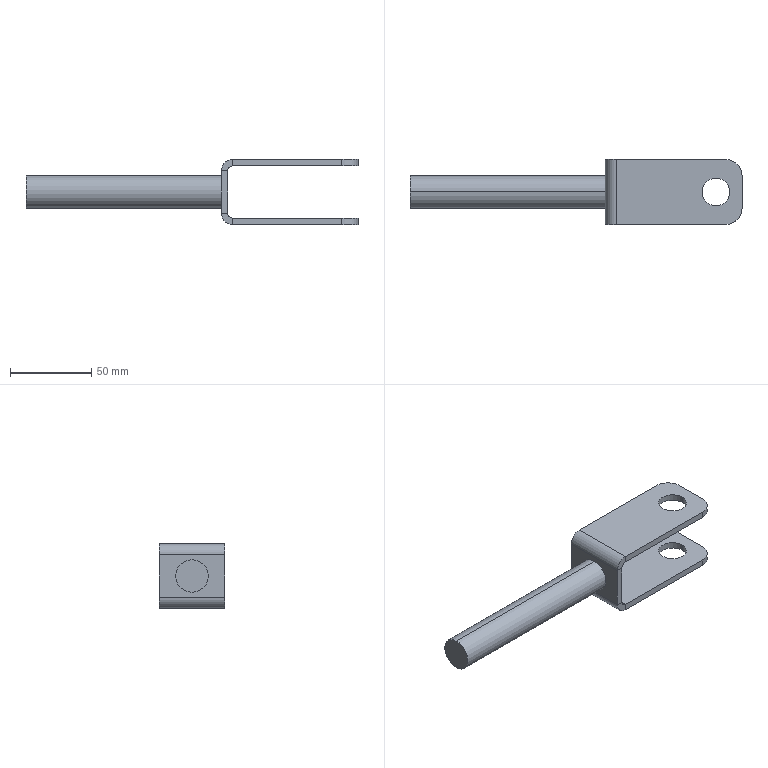Part | STEP file | TENSION_WHEEL1V11 | 1 solid | 33 faces | box 204 x 40 x 40 mm | volume 66853 mm3 | plane 19 | cylinder 14 | commonest cylinder face diameters 20 x6 17 x4 6 x2 14 x2